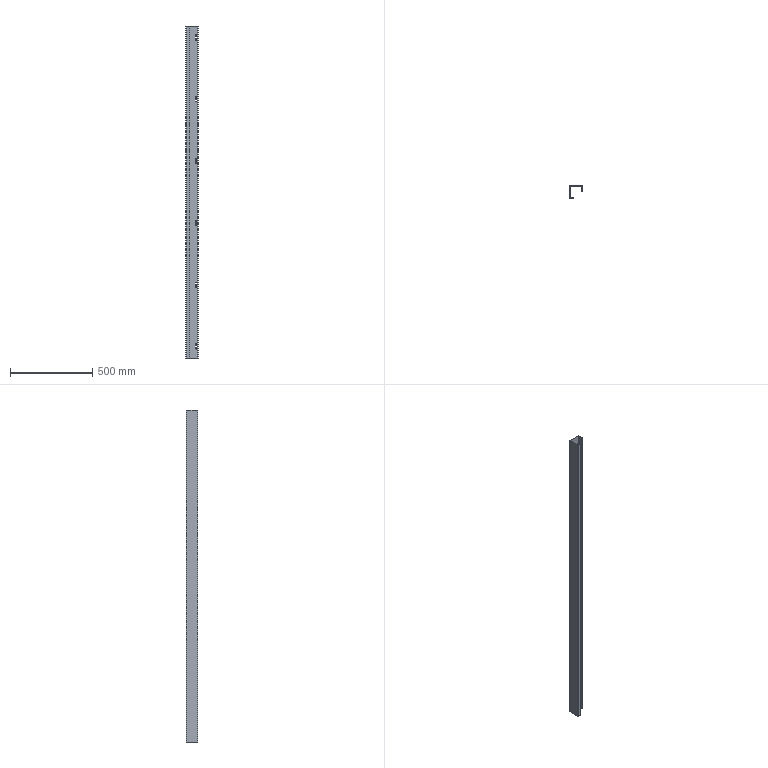Part | 1 solid | 60 faces | box 75 x 70 x 2016 mm | volume 457725 mm3 | plane 36 | cylinder 24 | commonest cylinder face diameters 9 x18 1 x3 3.4 x3